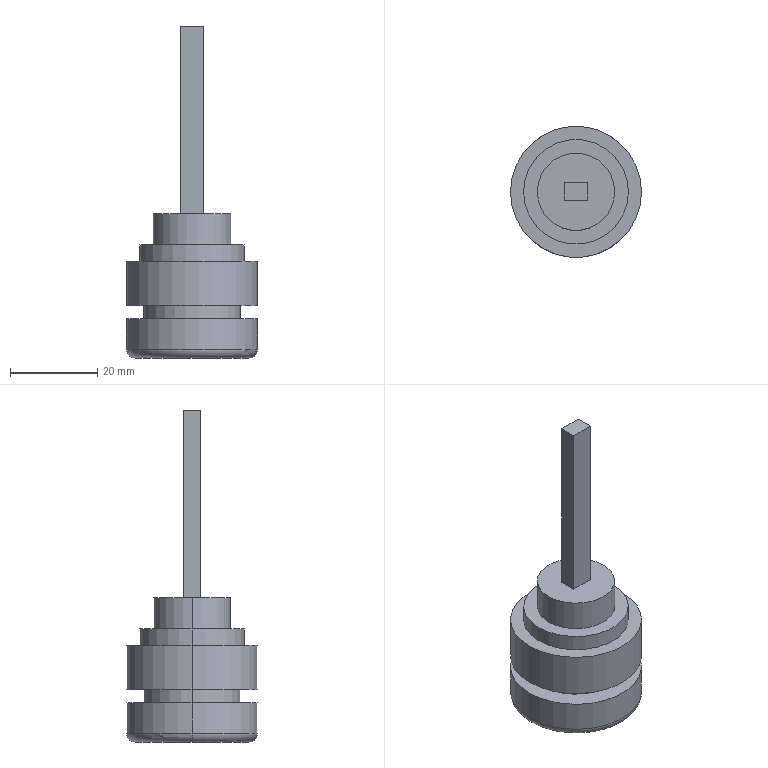Part | STEP file | Pushbutton head LA42PD-Y | 1 solid | 23 faces | box 30 x 30 x 76 mm | volume 18961 mm3 | plane 11 | cylinder 10 | torus 2 | commonest cylinder face diameters 30 x4 17.722 x2 22 x2 23.995 x2
STEP:
#1=CARTESIAN_POINT('',(0.,0.,0.));
#2=DIRECTION('',(0.,0.,1.));
#3=DIRECTION('',(1.,0.,0.));
#4=AXIS2_PLACEMENT_3D('',#1,#2,#3);
#5=CARTESIAN_POINT('',(13.,0.,0.));
#6=VERTEX_POINT('',#5);
#7=CARTESIAN_POINT('',(-13.,0.,0.));
#8=VERTEX_POINT('',#7);
#9=CARTESIAN_POINT('',(0.,0.,0.));
#10=DIRECTION('',(0.,0.,1.));
#11=DIRECTION('',(1.,0.,0.));
#12=AXIS2_PLACEMENT_3D('',#9,#10,#11);
#13=CIRCLE('',#12,13.);
#14=CARTESIAN_POINT('',(0.,0.,2.));
#15=DIRECTION('',(0.,0.,1.));
#16=DIRECTION('',(1.,0.,0.));
#17=AXIS2_PLACEMENT_3D('',#14,#15,#16);
#18=TOROIDAL_SURFACE('',#17,13.,2.);
#19=CARTESIAN_POINT('',(0.,4.712));
#20=DIRECTION('',(1.,0.));
#21=VECTOR('',#20,1.);
#22=LINE('',#19,#21);
#23=(GEOMETRIC_REPRESENTATION_CONTEXT(2)PARAMETRIC_REPRESENTATION_CONTEXT()REPRESENTATION_CONTEXT('',''));
#24=DEFINITIONAL_REPRESENTATION('',(#22),#23);
#25=PCURVE('',#18,#24);
#26=CARTESIAN_POINT('',(0.,0.,0.));
#27=DIRECTION('',(0.,0.,-1.));
#28=DIRECTION('',(-1.,0.,0.));
#29=AXIS2_PLACEMENT_3D('',#26,#27,#28);
#30=PLANE('',#29);
#31=CARTESIAN_POINT('',(-13.,0.));
#32=CARTESIAN_POINT('',(-13.,22.517));
#33=CARTESIAN_POINT('',(6.5,11.258));
#34=CARTESIAN_POINT('',(26.,0.));
#35=CARTESIAN_POINT('',(6.5,-11.258));
#36=CARTESIAN_POINT('',(-13.,-22.517));
#37=CARTESIAN_POINT('',(-13.,0.));
#38=(BOUNDED_CURVE()B_SPLINE_CURVE(2,(#31,#32,#33,#34,#35,#36,#37),.UNSPECIFIED.,.T.,.F.)B_SPLINE_CURVE_WITH_KNOTS((1,2,2,2,2,1),(-2.094,0.,2.094,4.189,6.283,8.378),.UNSPECIFIED.)CURVE()GEOMETRIC_REPRESENTATION_ITEM()RATIONAL_B_SPLINE_CURVE((1.,0.5,1.,0.5,1.,0.5,1.))REPRESENTATION_ITEM(''));
#39=(GEOMETRIC_REPRESENTATION_CONTEXT(2)PARAMETRIC_REPRESENTATION_CONTEXT()REPRESENTATION_CONTEXT('',''));
#40=DEFINITIONAL_REPRESENTATION('',(#38),#39);
#41=PCURVE('',#30,#40);
#42=SURFACE_CURVE('',#13,(#25,#41),.PCURVE_S1.);
#43=EDGE_CURVE('',#6,#8,#42,.T.);
#44=ORIENTED_EDGE('',*,*,#43,.T.);
#45=CARTESIAN_POINT('',(-15.,0.,2.));
#46=VERTEX_POINT('',#45);
#47=CARTESIAN_POINT('',(-13.,0.,2.));
#48=DIRECTION('',(0.,1.,0.));
#49=DIRECTION('',(-1.,0.,0.));
#50=AXIS2_PLACEMENT_3D('',#47,#48,#49);
#51=CIRCLE('',#50,2.);
#52=CARTESIAN_POINT('',(3.142,0.));
#53=DIRECTION('',(0.,1.));
#54=VECTOR('',#53,1.);
#55=LINE('',#52,#54);
#56=(GEOMETRIC_REPRESENTATION_CONTEXT(2)PARAMETRIC_REPRESENTATION_CONTEXT()REPRESENTATION_CONTEXT('',''));
#57=DEFINITIONAL_REPRESENTATION('',(#55),#56);
#58=PCURVE('',#18,#57);
#59=CARTESIAN_POINT('',(0.,0.,2.));
#60=DIRECTION('',(0.,0.,1.));
#61=DIRECTION('',(1.,0.,0.));
#62=AXIS2_PLACEMENT_3D('',#59,#60,#61);
#63=TOROIDAL_SURFACE('',#62,13.,2.);
#64=CARTESIAN_POINT('',(3.142,0.));
#65=DIRECTION('',(0.,1.));
#66=VECTOR('',#65,1.);
#67=LINE('',#64,#66);
#68=(GEOMETRIC_REPRESENTATION_CONTEXT(2)PARAMETRIC_REPRESENTATION_CONTEXT()REPRESENTATION_CONTEXT('',''));
#69=DEFINITIONAL_REPRESENTATION('',(#67),#68);
#70=PCURVE('',#63,#69);
#71=SURFACE_CURVE('',#51,(#58,#70),.PCURVE_S1.);
#72=EDGE_CURVE('',#8,#46,#71,.T.);
#73=ORIENTED_EDGE('',*,*,#72,.T.);
#74=CARTESIAN_POINT('',(15.,0.,2.));
#75=VERTEX_POINT('',#74);
#76=CARTESIAN_POINT('',(0.,0.,2.));
#77=DIRECTION('',(0.,0.,1.));
#78=DIRECTION('',(1.,0.,0.));
#79=AXIS2_PLACEMENT_3D('',#76,#77,#78);
#80=CIRCLE('',#79,15.);
#81=CARTESIAN_POINT('',(0.,6.283));
#82=DIRECTION('',(1.,0.));
#83=VECTOR('',#82,1.);
#84=LINE('',#81,#83);
#85=(GEOMETRIC_REPRESENTATION_CONTEXT(2)PARAMETRIC_REPRESENTATION_CONTEXT()REPRESENTATION_CONTEXT('',''));
#86=DEFINITIONAL_REPRESENTATION('',(#84),#85);
#87=PCURVE('',#18,#86);
#88=CARTESIAN_POINT('',(0.,0.,33.));
#89=DIRECTION('',(0.,0.,1.));
#90=DIRECTION('',(1.,0.,0.));
#91=AXIS2_PLACEMENT_3D('',#88,#89,#90);
#92=CYLINDRICAL_SURFACE('',#91,15.);
#93=CARTESIAN_POINT('',(0.,-31.));
#94=DIRECTION('',(1.,0.));
#95=VECTOR('',#94,1.);
#96=LINE('',#93,#95);
#97=(GEOMETRIC_REPRESENTATION_CONTEXT(2)PARAMETRIC_REPRESENTATION_CONTEXT()REPRESENTATION_CONTEXT('',''));
#98=DEFINITIONAL_REPRESENTATION('',(#96),#97);
#99=PCURVE('',#92,#98);
#100=SURFACE_CURVE('',#80,(#87,#99),.PCURVE_S1.);
#101=EDGE_CURVE('',#75,#46,#100,.T.);
#102=ORIENTED_EDGE('',*,*,#101,.F.);
#103=CARTESIAN_POINT('',(13.,0.,2.));
#104=DIRECTION('',(0.,-1.,0.));
#105=DIRECTION('',(0.,0.,-1.));
#106=AXIS2_PLACEMENT_3D('',#103,#104,#105);
#107=CIRCLE('',#106,2.);
#108=CARTESIAN_POINT('',(0.,4.712));
#109=DIRECTION('',(0.,1.));
#110=VECTOR('',#109,1.);
#111=LINE('',#108,#110);
#112=(GEOMETRIC_REPRESENTATION_CONTEXT(2)PARAMETRIC_REPRESENTATION_CONTEXT()REPRESENTATION_CONTEXT('',''));
#113=DEFINITIONAL_REPRESENTATION('',(#111),#112);
#114=PCURVE('',#18,#113);
#115=CARTESIAN_POINT('',(6.283,4.712));
#116=DIRECTION('',(0.,1.));
#117=VECTOR('',#116,1.);
#118=LINE('',#115,#117);
#119=(GEOMETRIC_REPRESENTATION_CONTEXT(2)PARAMETRIC_REPRESENTATION_CONTEXT()REPRESENTATION_CONTEXT('',''));
#120=DEFINITIONAL_REPRESENTATION('',(#118),#119);
#121=PCURVE('',#63,#120);
#122=SURFACE_CURVE('',#107,(#114,#121),.PCURVE_S1.);
#123=EDGE_CURVE('',#6,#75,#122,.T.);
#124=ORIENTED_EDGE('',*,*,#123,.F.);
#125=EDGE_LOOP('',(#44,#73,#102,#124));
#126=FACE_BOUND('',#125,.T.);
#127=ADVANCED_FACE('',(#126),#18,.T.);
#128=ORIENTED_EDGE('',*,*,#101,.T.);
#129=CARTESIAN_POINT('',(-15.,0.,9.));
#130=VERTEX_POINT('',#129);
#131=CARTESIAN_POINT('',(-15.,0.,33.));
#132=DIRECTION('',(0.,0.,1.));
#133=VECTOR('',#132,1.);
#134=LINE('',#131,#133);
#135=CARTESIAN_POINT('',(3.142,0.));
#136=DIRECTION('',(0.,1.));
#137=VECTOR('',#136,1.);
#138=LINE('',#135,#137);
#139=(GEOMETRIC_REPRESENTATION_CONTEXT(2)PARAMETRIC_REPRESENTATION_CONTEXT()REPRESENTATION_CONTEXT('',''));
#140=DEFINITIONAL_REPRESENTATION('',(#138),#139);
#141=PCURVE('',#92,#140);
#142=CARTESIAN_POINT('',(0.,0.,33.));
#143=DIRECTION('',(0.,0.,1.));
#144=DIRECTION('',(1.,0.,0.));
#145=AXIS2_PLACEMENT_3D('',#142,#143,#144);
#146=CYLINDRICAL_SURFACE('',#145,15.);
#147=CARTESIAN_POINT('',(3.142,0.));
#148=DIRECTION('',(0.,1.));
#149=VECTOR('',#148,1.);
#150=LINE('',#147,#149);
#151=(GEOMETRIC_REPRESENTATION_CONTEXT(2)PARAMETRIC_REPRESENTATION_CONTEXT()REPRESENTATION_CONTEXT('',''));
#152=DEFINITIONAL_REPRESENTATION('',(#150),#151);
#153=PCURVE('',#146,#152);
#154=SURFACE_CURVE('',#134,(#141,#153),.PCURVE_S1.);
#155=EDGE_CURVE('',#46,#130,#154,.T.);
#156=ORIENTED_EDGE('',*,*,#155,.T.);
#157=CARTESIAN_POINT('',(15.,0.,9.));
#158=VERTEX_POINT('',#157);
#159=CARTESIAN_POINT('',(0.,0.,9.));
#160=DIRECTION('',(0.,0.,1.));
#161=DIRECTION('',(1.,0.,0.));
#162=AXIS2_PLACEMENT_3D('',#159,#160,#161);
#163=CIRCLE('',#162,15.);
#164=CARTESIAN_POINT('',(0.,-24.));
#165=DIRECTION('',(1.,0.));
#166=VECTOR('',#165,1.);
#167=LINE('',#164,#166);
#168=(GEOMETRIC_REPRESENTATION_CONTEXT(2)PARAMETRIC_REPRESENTATION_CONTEXT()REPRESENTATION_CONTEXT('',''));
#169=DEFINITIONAL_REPRESENTATION('',(#167),#168);
#170=PCURVE('',#92,#169);
#171=CARTESIAN_POINT('',(15.,0.,9.));
#172=DIRECTION('',(0.,0.,1.));
#173=DIRECTION('',(1.,0.,0.));
#174=AXIS2_PLACEMENT_3D('',#171,#172,#173);
#175=PLANE('',#174);
#176=CARTESIAN_POINT('',(-15.,0.));
#177=DIRECTION('',(1.,0.));
#178=AXIS2_PLACEMENT_2D('',#176,#177);
#179=CIRCLE('',#178,15.);
#180=(GEOMETRIC_REPRESENTATION_CONTEXT(2)PARAMETRIC_REPRESENTATION_CONTEXT()REPRESENTATION_CONTEXT('',''));
#181=DEFINITIONAL_REPRESENTATION('',(#179),#180);
#182=PCURVE('',#175,#181);
#183=SURFACE_CURVE('',#163,(#170,#182),.PCURVE_S1.);
#184=EDGE_CURVE('',#158,#130,#183,.T.);
#185=ORIENTED_EDGE('',*,*,#184,.F.);
#186=CARTESIAN_POINT('',(15.,0.,33.));
#187=DIRECTION('',(0.,0.,1.));
#188=VECTOR('',#187,1.);
#189=LINE('',#186,#188);
#190=CARTESIAN_POINT('',(0.,0.));
#191=DIRECTION('',(0.,1.));
#192=VECTOR('',#191,1.);
#193=LINE('',#190,#192);
#194=(GEOMETRIC_REPRESENTATION_CONTEXT(2)PARAMETRIC_REPRESENTATION_CONTEXT()REPRESENTATION_CONTEXT('',''));
#195=DEFINITIONAL_REPRESENTATION('',(#193),#194);
#196=PCURVE('',#92,#195);
#197=CARTESIAN_POINT('',(6.283,0.));
#198=DIRECTION('',(0.,1.));
#199=VECTOR('',#198,1.);
#200=LINE('',#197,#199);
#201=(GEOMETRIC_REPRESENTATION_CONTEXT(2)PARAMETRIC_REPRESENTATION_CONTEXT()REPRESENTATION_CONTEXT('',''));
#202=DEFINITIONAL_REPRESENTATION('',(#200),#201);
#203=PCURVE('',#146,#202);
#204=SURFACE_CURVE('',#189,(#196,#203),.PCURVE_S1.);
#205=EDGE_CURVE('',#75,#158,#204,.T.);
#206=ORIENTED_EDGE('',*,*,#205,.F.);
#207=EDGE_LOOP('',(#128,#156,#185,#206));
#208=FACE_BOUND('',#207,.T.);
#209=ADVANCED_FACE('',(#208),#92,.T.);
#210=CARTESIAN_POINT('',(11.,0.,9.));
#211=VERTEX_POINT('',#210);
#212=CARTESIAN_POINT('',(-11.,0.,9.));
#213=VERTEX_POINT('',#212);
#214=CARTESIAN_POINT('',(0.,0.,9.));
#215=DIRECTION('',(0.,0.,1.));
#216=DIRECTION('',(1.,0.,0.));
#217=AXIS2_PLACEMENT_3D('',#214,#215,#216);
#218=CIRCLE('',#217,11.);
#219=CARTESIAN_POINT('',(0.,0.,33.));
#220=DIRECTION('',(0.,0.,1.));
#221=DIRECTION('',(1.,0.,0.));
#222=AXIS2_PLACEMENT_3D('',#219,#220,#221);
#223=CYLINDRICAL_SURFACE('',#222,11.);
#224=CARTESIAN_POINT('',(0.,-24.));
#225=DIRECTION('',(1.,0.));
#226=VECTOR('',#225,1.);
#227=LINE('',#224,#226);
#228=(GEOMETRIC_REPRESENTATION_CONTEXT(2)PARAMETRIC_REPRESENTATION_CONTEXT()REPRESENTATION_CONTEXT('',''));
#229=DEFINITIONAL_REPRESENTATION('',(#227),#228);
#230=PCURVE('',#223,#229);
#231=CARTESIAN_POINT('',(-15.,0.));
#232=DIRECTION('',(1.,0.));
#233=AXIS2_PLACEMENT_2D('',#231,#232);
#234=CIRCLE('',#233,11.);
#235=(GEOMETRIC_REPRESENTATION_CONTEXT(2)PARAMETRIC_REPRESENTATION_CONTEXT()REPRESENTATION_CONTEXT('',''));
#236=DEFINITIONAL_REPRESENTATION('',(#234),#235);
#237=PCURVE('',#175,#236);
#238=SURFACE_CURVE('',#218,(#230,#237),.PCURVE_S1.);
#239=EDGE_CURVE('',#211,#213,#238,.T.);
#240=ORIENTED_EDGE('',*,*,#239,.T.);
#241=CARTESIAN_POINT('',(-11.,0.,12.));
#242=VERTEX_POINT('',#241);
#243=CARTESIAN_POINT('',(-11.,0.,33.));
#244=DIRECTION('',(0.,0.,1.));
#245=VECTOR('',#244,1.);
#246=LINE('',#243,#245);
#247=CARTESIAN_POINT('',(3.142,0.));
#248=DIRECTION('',(0.,1.));
#249=VECTOR('',#248,1.);
#250=LINE('',#247,#249);
#251=(GEOMETRIC_REPRESENTATION_CONTEXT(2)PARAMETRIC_REPRESENTATION_CONTEXT()REPRESENTATION_CONTEXT('',''));
#252=DEFINITIONAL_REPRESENTATION('',(#250),#251);
#253=PCURVE('',#223,#252);
#254=CARTESIAN_POINT('',(0.,0.,33.));
#255=DIRECTION('',(0.,0.,1.));
#256=DIRECTION('',(1.,0.,0.));
#257=AXIS2_PLACEMENT_3D('',#254,#255,#256);
#258=CYLINDRICAL_SURFACE('',#257,11.);
#259=CARTESIAN_POINT('',(3.142,0.));
#260=DIRECTION('',(0.,1.));
#261=VECTOR('',#260,1.);
#262=LINE('',#259,#261);
#263=(GEOMETRIC_REPRESENTATION_CONTEXT(2)PARAMETRIC_REPRESENTATION_CONTEXT()REPRESENTATION_CONTEXT('',''));
#264=DEFINITIONAL_REPRESENTATION('',(#262),#263);
#265=PCURVE('',#258,#264);
#266=SURFACE_CURVE('',#246,(#253,#265),.PCURVE_S1.);
#267=EDGE_CURVE('',#213,#242,#266,.T.);
#268=ORIENTED_EDGE('',*,*,#267,.T.);
#269=CARTESIAN_POINT('',(11.,0.,12.));
#270=VERTEX_POINT('',#269);
#271=CARTESIAN_POINT('',(0.,0.,12.));
#272=DIRECTION('',(0.,0.,1.));
#273=DIRECTION('',(1.,0.,0.));
#274=AXIS2_PLACEMENT_3D('',#271,#272,#273);
#275=CIRCLE('',#274,11.);
#276=CARTESIAN_POINT('',(0.,-21.));
#277=DIRECTION('',(1.,0.));
#278=VECTOR('',#277,1.);
#279=LINE('',#276,#278);
#280=(GEOMETRIC_REPRESENTATION_CONTEXT(2)PARAMETRIC_REPRESENTATION_CONTEXT()REPRESENTATION_CONTEXT('',''));
#281=DEFINITIONAL_REPRESENTATION('',(#279),#280);
#282=PCURVE('',#223,#281);
#283=CARTESIAN_POINT('',(11.,0.,12.));
#284=DIRECTION('',(0.,0.,-1.));
#285=DIRECTION('',(-1.,0.,0.));
#286=AXIS2_PLACEMENT_3D('',#283,#284,#285);
#287=PLANE('',#286);
#288=CARTESIAN_POINT('',(0.,0.));
#289=CARTESIAN_POINT('',(0.,19.053));
#290=CARTESIAN_POINT('',(16.5,9.526));
#291=CARTESIAN_POINT('',(33.,0.));
#292=CARTESIAN_POINT('',(16.5,-9.526));
#293=CARTESIAN_POINT('',(0.,-19.053));
#294=CARTESIAN_POINT('',(0.,0.));
#295=(BOUNDED_CURVE()B_SPLINE_CURVE(2,(#288,#289,#290,#291,#292,#293,#294),.UNSPECIFIED.,.T.,.F.)B_SPLINE_CURVE_WITH_KNOTS((1,2,2,2,2,1),(-2.094,0.,2.094,4.189,6.283,8.378),.UNSPECIFIED.)CURVE()GEOMETRIC_REPRESENTATION_ITEM()RATIONAL_B_SPLINE_CURVE((1.,0.5,1.,0.5,1.,0.5,1.))REPRESENTATION_ITEM(''));
#296=(GEOMETRIC_REPRESENTATION_CONTEXT(2)PARAMETRIC_REPRESENTATION_CONTEXT()REPRESENTATION_CONTEXT('',''));
#297=DEFINITIONAL_REPRESENTATION('',(#295),#296);
#298=PCURVE('',#287,#297);
#299=SURFACE_CURVE('',#275,(#282,#298),.PCURVE_S1.);
#300=EDGE_CURVE('',#270,#242,#299,.T.);
#301=ORIENTED_EDGE('',*,*,#300,.F.);
#302=CARTESIAN_POINT('',(11.,0.,33.));
#303=DIRECTION('',(0.,0.,1.));
#304=VECTOR('',#303,1.);
#305=LINE('',#302,#304);
#306=CARTESIAN_POINT('',(0.,0.));
#307=DIRECTION('',(0.,1.));
#308=VECTOR('',#307,1.);
#309=LINE('',#306,#308);
#310=(GEOMETRIC_REPRESENTATION_CONTEXT(2)PARAMETRIC_REPRESENTATION_CONTEXT()REPRESENTATION_CONTEXT('',''));
#311=DEFINITIONAL_REPRESENTATION('',(#309),#310);
#312=PCURVE('',#223,#311);
#313=CARTESIAN_POINT('',(6.283,0.));
#314=DIRECTION('',(0.,1.));
#315=VECTOR('',#314,1.);
#316=LINE('',#313,#315);
#317=(GEOMETRIC_REPRESENTATION_CONTEXT(2)PARAMETRIC_REPRESENTATION_CONTEXT()REPRESENTATION_CONTEXT('',''));
#318=DEFINITIONAL_REPRESENTATION('',(#316),#317);
#319=PCURVE('',#258,#318);
#320=SURFACE_CURVE('',#305,(#312,#319),.PCURVE_S1.);
#321=EDGE_CURVE('',#211,#270,#320,.T.);
#322=ORIENTED_EDGE('',*,*,#321,.F.);
#323=EDGE_LOOP('',(#240,#268,#301,#322));
#324=FACE_BOUND('',#323,.T.);
#325=ADVANCED_FACE('',(#324),#223,.T.);
#326=CARTESIAN_POINT('',(15.,0.,12.));
#327=VERTEX_POINT('',#326);
#328=CARTESIAN_POINT('',(-15.,0.,12.));
#329=VERTEX_POINT('',#328);
#330=CARTESIAN_POINT('',(0.,0.,12.));
#331=DIRECTION('',(0.,0.,1.));
#332=DIRECTION('',(1.,0.,0.));
#333=AXIS2_PLACEMENT_3D('',#330,#331,#332);
#334=CIRCLE('',#333,15.);
#335=CARTESIAN_POINT('',(0.,0.,33.));
#336=DIRECTION('',(0.,0.,1.));
#337=DIRECTION('',(1.,0.,0.));
#338=AXIS2_PLACEMENT_3D('',#335,#336,#337);
#339=CYLINDRICAL_SURFACE('',#338,15.);
#340=CARTESIAN_POINT('',(0.,-21.));
#341=DIRECTION('',(1.,0.));
#342=VECTOR('',#341,1.);
#343=LINE('',#340,#342);
#344=(GEOMETRIC_REPRESENTATION_CONTEXT(2)PARAMETRIC_REPRESENTATION_CONTEXT()REPRESENTATION_CONTEXT('',''));
#345=DEFINITIONAL_REPRESENTATION('',(#343),#344);
#346=PCURVE('',#339,#345);
#347=CARTESIAN_POINT('',(-4.,0.));
#348=CARTESIAN_POINT('',(-4.,25.981));
#349=CARTESIAN_POINT('',(18.5,12.99));
#350=CARTESIAN_POINT('',(41.,0.));
#351=CARTESIAN_POINT('',(18.5,-12.99));
#352=CARTESIAN_POINT('',(-4.,-25.981));
#353=CARTESIAN_POINT('',(-4.,0.));
#354=(BOUNDED_CURVE()B_SPLINE_CURVE(2,(#347,#348,#349,#350,#351,#352,#353),.UNSPECIFIED.,.T.,.F.)B_SPLINE_CURVE_WITH_KNOTS((1,2,2,2,2,1),(-2.094,0.,2.094,4.189,6.283,8.378),.UNSPECIFIED.)CURVE()GEOMETRIC_REPRESENTATION_ITEM()RATIONAL_B_SPLINE_CURVE((1.,0.5,1.,0.5,1.,0.5,1.))REPRESENTATION_ITEM(''));
#355=(GEOMETRIC_REPRESENTATION_CONTEXT(2)PARAMETRIC_REPRESENTATION_CONTEXT()REPRESENTATION_CONTEXT('',''));
#356=DEFINITIONAL_REPRESENTATION('',(#354),#355);
#357=PCURVE('',#287,#356);
#358=SURFACE_CURVE('',#334,(#346,#357),.PCURVE_S1.);
#359=EDGE_CURVE('',#327,#329,#358,.T.);
#360=ORIENTED_EDGE('',*,*,#359,.T.);
#361=CARTESIAN_POINT('',(-15.,0.,22.166));
#362=VERTEX_POINT('',#361);
#363=CARTESIAN_POINT('',(-15.,0.,33.));
#364=DIRECTION('',(0.,0.,1.));
#365=VECTOR('',#364,1.);
#366=LINE('',#363,#365);
#367=CARTESIAN_POINT('',(3.142,0.));
#368=DIRECTION('',(0.,1.));
#369=VECTOR('',#368,1.);
#370=LINE('',#367,#369);
#371=(GEOMETRIC_REPRESENTATION_CONTEXT(2)PARAMETRIC_REPRESENTATION_CONTEXT()REPRESENTATION_CONTEXT('',''));
#372=DEFINITIONAL_REPRESENTATION('',(#370),#371);
#373=PCURVE('',#339,#372);
#374=CARTESIAN_POINT('',(0.,0.,33.));
#375=DIRECTION('',(0.,0.,1.));
#376=DIRECTION('',(1.,0.,0.));
#377=AXIS2_PLACEMENT_3D('',#374,#375,#376);
#378=CYLINDRICAL_SURFACE('',#377,15.);
#379=CARTESIAN_POINT('',(3.142,0.));
#380=DIRECTION('',(0.,1.));
#381=VECTOR('',#380,1.);
#382=LINE('',#379,#381);
#383=(GEOMETRIC_REPRESENTATION_CONTEXT(2)PARAMETRIC_REPRESENTATION_CONTEXT()REPRESENTATION_CONTEXT('',''));
#384=DEFINITIONAL_REPRESENTATION('',(#382),#383);
#385=PCURVE('',#378,#384);
#386=SURFACE_CURVE('',#366,(#373,#385),.PCURVE_S1.);
#387=EDGE_CURVE('',#329,#362,#386,.T.);
#388=ORIENTED_EDGE('',*,*,#387,.T.);
#389=CARTESIAN_POINT('',(15.,0.,22.166));
#390=VERTEX_POINT('',#389);
#391=CARTESIAN_POINT('',(0.,0.,22.166));
#392=DIRECTION('',(0.,0.,1.));
#393=DIRECTION('',(1.,0.,0.));
#394=AXIS2_PLACEMENT_3D('',#391,#392,#393);
#395=CIRCLE('',#394,15.);
#396=CARTESIAN_POINT('',(0.,-10.834));
#397=DIRECTION('',(1.,0.));
#398=VECTOR('',#397,1.);
#399=LINE('',#396,#398);
#400=(GEOMETRIC_REPRESENTATION_CONTEXT(2)PARAMETRIC_REPRESENTATION_CONTEXT()REPRESENTATION_CONTEXT('',''));
#401=DEFINITIONAL_REPRESENTATION('',(#399),#400);
#402=PCURVE('',#339,#401);
#403=CARTESIAN_POINT('',(15.,0.,22.166));
#404=DIRECTION('',(0.,0.,1.));
#405=DIRECTION('',(1.,0.,0.));
#406=AXIS2_PLACEMENT_3D('',#403,#404,#405);
#407=PLANE('',#406);
#408=CARTESIAN_POINT('',(-15.,0.));
#409=DIRECTION('',(1.,0.));
#410=AXIS2_PLACEMENT_2D('',#408,#409);
#411=CIRCLE('',#410,15.);
#412=(GEOMETRIC_REPRESENTATION_CONTEXT(2)PARAMETRIC_REPRESENTATION_CONTEXT()REPRESENTATION_CONTEXT('',''));
#413=DEFINITIONAL_REPRESENTATION('',(#411),#412);
#414=PCURVE('',#407,#413);
#415=SURFACE_CURVE('',#395,(#402,#414),.PCURVE_S1.);
#416=EDGE_CURVE('',#390,#362,#415,.T.);
#417=ORIENTED_EDGE('',*,*,#416,.F.);
#418=CARTESIAN_POINT('',(15.,0.,33.));
#419=DIRECTION('',(0.,0.,1.));
#420=VECTOR('',#419,1.);
#421=LINE('',#418,#420);
#422=CARTESIAN_POINT('',(0.,0.));
#423=DIRECTION('',(0.,1.));
#424=VECTOR('',#423,1.);
#425=LINE('',#422,#424);
#426=(GEOMETRIC_REPRESENTATION_CONTEXT(2)PARAMETRIC_REPRESENTATION_CONTEXT()REPRESENTATION_CONTEXT('',''));
#427=DEFINITIONAL_REPRESENTATION('',(#425),#426);
#428=PCURVE('',#339,#427);
#429=CARTESIAN_POINT('',(6.283,0.));
#430=DIRECTION('',(0.,1.));
#431=VECTOR('',#430,1.);
#432=LINE('',#429,#431);
#433=(GEOMETRIC_REPRESENTATION_CONTEXT(2)PARAMETRIC_REPRESENTATION_CONTEXT()REPRESENTATION_CONTEXT('',''));
#434=DEFINITIONAL_REPRESENTATION('',(#432),#433);
#435=PCURVE('',#378,#434);
#436=SURFACE_CURVE('',#421,(#428,#435),.PCURVE_S1.);
#437=EDGE_CURVE('',#327,#390,#436,.T.);
#438=ORIENTED_EDGE('',*,*,#437,.F.);
#439=EDGE_LOOP('',(#360,#388,#417,#438));
#440=FACE_BOUND('',#439,.T.);
#441=ADVANCED_FACE('',(#440),#339,.T.);
#442=CARTESIAN_POINT('',(11.997,0.,22.166));
#443=VERTEX_POINT('',#442);
#444=CARTESIAN_POINT('',(-11.997,0.,22.166));
#445=VERTEX_POINT('',#444);
#446=CARTESIAN_POINT('',(0.,0.,22.166));
#447=DIRECTION('',(0.,0.,1.));
#448=DIRECTION('',(1.,0.,0.));
#449=AXIS2_PLACEMENT_3D('',#446,#447,#448);
#450=CIRCLE('',#449,11.997);
#451=CARTESIAN_POINT('',(0.,0.,33.));
#452=DIRECTION('',(0.,0.,1.));
#453=DIRECTION('',(1.,0.,0.));
#454=AXIS2_PLACEMENT_3D('',#451,#452,#453);
#455=CYLINDRICAL_SURFACE('',#454,11.997);
#456=CARTESIAN_POINT('',(0.,-10.834));
#457=DIRECTION('',(1.,0.));
#458=VECTOR('',#457,1.);
#459=LINE('',#456,#458);
#460=(GEOMETRIC_REPRESENTATION_CONTEXT(2)PARAMETRIC_REPRESENTATION_CONTEXT()REPRESENTATION_CONTEXT('',''));
#461=DEFINITIONAL_REPRESENTATION('',(#459),#460);
#462=PCURVE('',#455,#461);
#463=CARTESIAN_POINT('',(-15.,0.));
#464=DIRECTION('',(1.,0.));
#465=AXIS2_PLACEMENT_2D('',#463,#464);
#466=CIRCLE('',#465,11.997);
#467=(GEOMETRIC_REPRESENTATION_CONTEXT(2)PARAMETRIC_REPRESENTATION_CONTEXT()REPRESENTATION_CONTEXT('',''));
#468=DEFINITIONAL_REPRESENTATION('',(#466),#467);
#469=PCURVE('',#407,#468);
#470=SURFACE_CURVE('',#450,(#462,#469),.PCURVE_S1.);
#471=EDGE_CURVE('',#443,#445,#470,.T.);
#472=ORIENTED_EDGE('',*,*,#471,.T.);
#473=CARTESIAN_POINT('',(-11.997,0.,25.869));
#474=VERTEX_POINT('',#473);
#475=CARTESIAN_POINT('',(-11.997,0.,33.));
#476=DIRECTION('',(0.,0.,1.));
#477=VECTOR('',#476,1.);
#478=LINE('',#475,#477);
#479=CARTESIAN_POINT('',(3.142,0.));
#480=DIRECTION('',(0.,1.));
#481=VECTOR('',#480,1.);
#482=LINE('',#479,#481);
#483=(GEOMETRIC_REPRESENTATION_CONTEXT(2)PARAMETRIC_REPRESENTATION_CONTEXT()REPRESENTATION_CONTEXT('',''));
#484=DEFINITIONAL_REPRESENTATION('',(#482),#483);
#485=PCURVE('',#455,#484);
#486=CARTESIAN_POINT('',(0.,0.,33.));
#487=DIRECTION('',(0.,0.,1.));
#488=DIRECTION('',(1.,0.,0.));
#489=AXIS2_PLACEMENT_3D('',#486,#487,#488);
#490=CYLINDRICAL_SURFACE('',#489,11.997);
#491=CARTESIAN_POINT('',(3.142,0.));
#492=DIRECTION('',(0.,1.));
#493=VECTOR('',#492,1.);
#494=LINE('',#491,#493);
#495=(GEOMETRIC_REPRESENTATION_CONTEXT(2)PARAMETRIC_REPRESENTATION_CONTEXT()REPRESENTATION_CONTEXT('',''));
#496=DEFINITIONAL_REPRESENTATION('',(#494),#495);
#497=PCURVE('',#490,#496);
#498=SURFACE_CURVE('',#478,(#485,#497),.PCURVE_S1.);
#499=EDGE_CURVE('',#445,#474,#498,.T.);
#500=ORIENTED_EDGE('',*,*,#499,.T.);
#501=CARTESIAN_POINT('',(11.997,0.,25.869));
#502=VERTEX_POINT('',#501);
#503=CARTESIAN_POINT('',(0.,0.,25.869));
#504=DIRECTION('',(0.,0.,1.));
#505=DIRECTION('',(1.,0.,0.));
#506=AXIS2_PLACEMENT_3D('',#503,#504,#505);
#507=CIRCLE('',#506,11.997);
#508=CARTESIAN_POINT('',(0.,-7.131));
#509=DIRECTION('',(1.,0.));
#510=VECTOR('',#509,1.);
#511=LINE('',#508,#510);
#512=(GEOMETRIC_REPRESENTATION_CONTEXT(2)PARAMETRIC_REPRESENTATION_CONTEXT()REPRESENTATION_CONTEXT('',''));
#513=DEFINITIONAL_REPRESENTATION('',(#511),#512);
#514=PCURVE('',#455,#513);
#515=CARTESIAN_POINT('',(11.997,0.,25.869));
#516=DIRECTION('',(0.,0.,1.));
#517=DIRECTION('',(1.,0.,0.));
#518=AXIS2_PLACEMENT_3D('',#515,#516,#517);
#519=PLANE('',#518);
#520=CARTESIAN_POINT('',(-11.997,0.));
#521=DIRECTION('',(1.,0.));
#522=AXIS2_PLACEMENT_2D('',#520,#521);
#523=CIRCLE('',#522,11.997);
#524=(GEOMETRIC_REPRESENTATION_CONTEXT(2)PARAMETRIC_REPRESENTATION_CONTEXT()REPRESENTATION_CONTEXT('',''));
#525=DEFINITIONAL_REPRESENTATION('',(#523),#524);
#526=PCURVE('',#519,#525);
#527=SURFACE_CURVE('',#507,(#514,#526),.PCURVE_S1.);
#528=EDGE_CURVE('',#502,#474,#527,.T.);
#529=ORIENTED_EDGE('',*,*,#528,.F.);
#530=CARTESIAN_POINT('',(11.997,0.,33.));
#531=DIRECTION('',(0.,0.,1.));
#532=VECTOR('',#531,1.);
#533=LINE('',#530,#532);
#534=CARTESIAN_POINT('',(0.,0.));
#535=DIRECTION('',(0.,1.));
#536=VECTOR('',#535,1.);
#537=LINE('',#534,#536);
#538=(GEOMETRIC_REPRESENTATION_CONTEXT(2)PARAMETRIC_REPRESENTATION_CONTEXT()REPRESENTATION_CONTEXT('',''));
#539=DEFINITIONAL_REPRESENTATION('',(#537),#538);
#540=PCURVE('',#455,#539);
#541=CARTESIAN_POINT('',(6.283,0.));
#542=DIRECTION('',(0.,1.));
#543=VECTOR('',#542,1.);
#544=LINE('',#541,#543);
#545=(GEOMETRIC_REPRESENTATION_CONTEXT(2)PARAMETRIC_REPRESENTATION_CONTEXT()REPRESENTATION_CONTEXT('',''));
#546=DEFINITIONAL_REPRESENTATION('',(#544),#545);
#547=PCURVE('',#490,#546);
#548=SURFACE_CURVE('',#533,(#540,#547),.PCURVE_S1.);
#549=EDGE_CURVE('',#443,#502,#548,.T.);
#550=ORIENTED_EDGE('',*,*,#549,.F.);
#551=EDGE_LOOP('',(#472,#500,#529,#550));
#552=FACE_BOUND('',#551,.T.);
#553=ADVANCED_FACE('',(#552),#455,.T.);
#554=CARTESIAN_POINT('',(8.861,0.,25.869));
#555=VERTEX_POINT('',#554);
#556=CARTESIAN_POINT('',(-8.861,0.,25.869));
#557=VERTEX_POINT('',#556);
#558=CARTESIAN_POINT('',(0.,0.,25.869));
#559=DIRECTION('',(0.,0.,1.));
#560=DIRECTION('',(1.,0.,0.));
#561=AXIS2_PLACEMENT_3D('',#558,#559,#560);
#562=CIRCLE('',#561,8.861);
#563=CARTESIAN_POINT('',(0.,0.,33.));
#564=DIRECTION('',(0.,0.,1.));
#565=DIRECTION('',(1.,0.,0.));
#566=AXIS2_PLACEMENT_3D('',#563,#564,#565);
#567=CYLINDRICAL_SURFACE('',#566,8.861);
#568=CARTESIAN_POINT('',(0.,-7.131));
#569=DIRECTION('',(1.,0.));
#570=VECTOR('',#569,1.);
#571=LINE('',#568,#570);
#572=(GEOMETRIC_REPRESENTATION_CONTEXT(2)PARAMETRIC_REPRESENTATION_CONTEXT()REPRESENTATION_CONTEXT('',''));
#573=DEFINITIONAL_REPRESENTATION('',(#571),#572);
#574=PCURVE('',#567,#573);
#575=CARTESIAN_POINT('',(-11.997,0.));
#576=DIRECTION('',(1.,0.));
#577=AXIS2_PLACEMENT_2D('',#575,#576);
#578=CIRCLE('',#577,8.861);
#579=(GEOMETRIC_REPRESENTATION_CONTEXT(2)PARAMETRIC_REPRESENTATION_CONTEXT()REPRESENTATION_CONTEXT('',''));
#580=DEFINITIONAL_REPRESENTATION('',(#578),#579);
#581=PCURVE('',#519,#580);
#582=SURFACE_CURVE('',#562,(#574,#581),.PCURVE_S1.);
#583=EDGE_CURVE('',#555,#557,#582,.T.);
#584=ORIENTED_EDGE('',*,*,#583,.T.);
#585=CARTESIAN_POINT('',(-8.861,0.,33.));
#586=VERTEX_POINT('',#585);
#587=CARTESIAN_POINT('',(-8.861,0.,33.));
#588=DIRECTION('',(0.,0.,1.));
#589=VECTOR('',#588,1.);
#590=LINE('',#587,#589);
#591=CARTESIAN_POINT('',(3.142,0.));
#592=DIRECTION('',(0.,1.));
#593=VECTOR('',#592,1.);
#594=LINE('',#591,#593);
#595=(GEOMETRIC_REPRESENTATION_CONTEXT(2)PARAMETRIC_REPRESENTATION_CONTEXT()REPRESENTATION_CONTEXT('',''));
#596=DEFINITIONAL_REPRESENTATION('',(#594),#595);
#597=PCURVE('',#567,#596);
#598=CARTESIAN_POINT('',(0.,0.,33.));
#599=DIRECTION('',(0.,0.,1.));
#600=DIRECTION('',(1.,0.,0.));
#601=AXIS2_PLACEMENT_3D('',#598,#599,#600);
#602=CYLINDRICAL_SURFACE('',#601,8.861);
#603=CARTESIAN_POINT('',(3.142,0.));
#604=DIRECTION('',(0.,1.));
#605=VECTOR('',#604,1.);
#606=LINE('',#603,#605);
#607=(GEOMETRIC_REPRESENTATION_CONTEXT(2)PARAMETRIC_REPRESENTATION_CONTEXT()REPRESENTATION_CONTEXT('',''));
#608=DEFINITIONAL_REPRESENTATION('',(#606),#607);
#609=PCURVE('',#602,#608);
#610=SURFACE_CURVE('',#590,(#597,#609),.PCURVE_S1.);
#611=EDGE_CURVE('',#557,#586,#610,.T.);
#612=ORIENTED_EDGE('',*,*,#611,.T.);
#613=CARTESIAN_POINT('',(8.861,0.,33.));
#614=VERTEX_POINT('',#613);
#615=CARTESIAN_POINT('',(0.,0.,33.));
#616=DIRECTION('',(0.,0.,1.));
#617=DIRECTION('',(1.,0.,0.));
#618=AXIS2_PLACEMENT_3D('',#615,#616,#617);
#619=CIRCLE('',#618,8.861);
#620=CARTESIAN_POINT('',(0.,0.));
#621=DIRECTION('',(1.,0.));
#622=VECTOR('',#621,1.);
#623=LINE('',#620,#622);
#624=(GEOMETRIC_REPRESENTATION_CONTEXT(2)PARAMETRIC_REPRESENTATION_CONTEXT()REPRESENTATION_CONTEXT('',''));
#625=DEFINITIONAL_REPRESENTATION('',(#623),#624);
#626=PCURVE('',#567,#625);
#627=CARTESIAN_POINT('',(8.861,0.,33.));
#628=DIRECTION('',(0.,0.,1.));
#629=DIRECTION('',(1.,0.,0.));
#630=AXIS2_PLACEMENT_3D('',#627,#628,#629);
#631=PLANE('',#630);
#632=CARTESIAN_POINT('',(-8.861,0.));
#633=DIRECTION('',(1.,0.));
#634=AXIS2_PLACEMENT_2D('',#632,#633);
#635=CIRCLE('',#634,8.861);
#636=(GEOMETRIC_REPRESENTATION_CONTEXT(2)PARAMETRIC_REPRESENTATION_CONTEXT()REPRESENTATION_CONTEXT('',''));
#637=DEFINITIONAL_REPRESENTATION('',(#635),#636);
#638=PCURVE('',#631,#637);
#639=SURFACE_CURVE('',#619,(#626,#638),.PCURVE_S1.);
#640=EDGE_CURVE('',#614,#586,#639,.T.);
#641=ORIENTED_EDGE('',*,*,#640,.F.);
#642=CARTESIAN_POINT('',(8.861,0.,33.));
#643=DIRECTION('',(0.,0.,1.));
#644=VECTOR('',#643,1.);
#645=LINE('',#642,#644);
#646=CARTESIAN_POINT('',(0.,0.));
#647=DIRECTION('',(0.,1.));
#648=VECTOR('',#647,1.);
#649=LINE('',#646,#648);
#650=(GEOMETRIC_REPRESENTATION_CONTEXT(2)PARAMETRIC_REPRESENTATION_CONTEXT()REPRESENTATION_CONTEXT('',''));
#651=DEFINITIONAL_REPRESENTATION('',(#649),#650);
#652=PCURVE('',#567,#651);
#653=CARTESIAN_POINT('',(6.283,0.));
#654=DIRECTION('',(0.,1.));
#655=VECTOR('',#654,1.);
#656=LINE('',#653,#655);
#657=(GEOMETRIC_REPRESENTATION_CONTEXT(2)PARAMETRIC_REPRESENTATION_CONTEXT()REPRESENTATION_CONTEXT('',''));
#658=DEFINITIONAL_REPRESENTATION('',(#656),#657);
#659=PCURVE('',#602,#658);
#660=SURFACE_CURVE('',#645,(#652,#659),.PCURVE_S1.);
#661=EDGE_CURVE('',#555,#614,#660,.T.);
#662=ORIENTED_EDGE('',*,*,#661,.F.);
#663=EDGE_LOOP('',(#584,#612,#641,#662));
#664=FACE_BOUND('',#663,.T.);
#665=ADVANCED_FACE('',(#664),#567,.T.);
#666=ORIENTED_EDGE('',*,*,#640,.T.);
#667=CARTESIAN_POINT('',(0.,0.,33.));
#668=DIRECTION('',(0.,0.,1.));
#669=DIRECTION('',(1.,0.,0.));
#670=AXIS2_PLACEMENT_3D('',#667,#668,#669);
#671=CIRCLE('',#670,8.861);
#672=CARTESIAN_POINT('',(-8.861,0.));
#673=DIRECTION('',(1.,0.));
#674=AXIS2_PLACEMENT_2D('',#672,#673);
#675=CIRCLE('',#674,8.861);
#676=(GEOMETRIC_REPRESENTATION_CONTEXT(2)PARAMETRIC_REPRESENTATION_CONTEXT()REPRESENTATION_CONTEXT('',''));
#677=DEFINITIONAL_REPRESENTATION('',(#675),#676);
#678=PCURVE('',#631,#677);
#679=CARTESIAN_POINT('',(0.,0.));
#680=DIRECTION('',(1.,0.));
#681=VECTOR('',#680,1.);
#682=LINE('',#679,#681);
#683=(GEOMETRIC_REPRESENTATION_CONTEXT(2)PARAMETRIC_REPRESENTATION_CONTEXT()REPRESENTATION_CONTEXT('',''));
#684=DEFINITIONAL_REPRESENTATION('',(#682),#683);
#685=PCURVE('',#602,#684);
#686=SURFACE_CURVE('',#671,(#678,#685),.PCURVE_S1.);
#687=EDGE_CURVE('',#586,#614,#686,.T.);
#688=ORIENTED_EDGE('',*,*,#687,.T.);
#689=EDGE_LOOP('',(#666,#688));
#690=FACE_BOUND('',#689,.T.);
#691=CARTESIAN_POINT('',(-2.708,1.971,33.));
#692=VERTEX_POINT('',#691);
#693=CARTESIAN_POINT('',(2.708,1.971,33.));
#694=VERTEX_POINT('',#693);
#695=CARTESIAN_POINT('',(8.861,1.971,33.));
#696=DIRECTION('',(1.,0.,0.));
#697=VECTOR('',#696,1.);
#698=LINE('',#695,#697);
#699=CARTESIAN_POINT('',(0.,1.971));
#700=DIRECTION('',(1.,0.));
#701=VECTOR('',#700,1.);
#702=LINE('',#699,#701);
#703=(GEOMETRIC_REPRESENTATION_CONTEXT(2)PARAMETRIC_REPRESENTATION_CONTEXT()REPRESENTATION_CONTEXT('',''));
#704=DEFINITIONAL_REPRESENTATION('',(#702),#703);
#705=PCURVE('',#631,#704);
#706=CARTESIAN_POINT('',(-2.708,1.971,76.));
#707=DIRECTION('',(0.,-1.,0.));
#708=DIRECTION('',(0.,0.,-1.));
#709=AXIS2_PLACEMENT_3D('',#706,#707,#708);
#710=PLANE('',#709);
#711=CARTESIAN_POINT('',(43.,11.569));
#712=DIRECTION('',(0.,1.));
#713=VECTOR('',#712,1.);
#714=LINE('',#711,#713);
#715=(GEOMETRIC_REPRESENTATION_CONTEXT(2)PARAMETRIC_REPRESENTATION_CONTEXT()REPRESENTATION_CONTEXT('',''));
#716=DEFINITIONAL_REPRESENTATION('',(#714),#715);
#717=PCURVE('',#710,#716);
#718=SURFACE_CURVE('',#698,(#705,#717),.PCURVE_S1.);
#719=EDGE_CURVE('',#692,#694,#718,.T.);
#720=ORIENTED_EDGE('',*,*,#719,.T.);
#721=CARTESIAN_POINT('',(2.708,-1.971,33.));
#722=VERTEX_POINT('',#721);
#723=CARTESIAN_POINT('',(2.708,0.,33.));
#724=DIRECTION('',(0.,-1.,0.));
#725=VECTOR('',#724,1.);
#726=LINE('',#723,#725);
#727=CARTESIAN_POINT('',(-6.153,0.));
#728=DIRECTION('',(0.,-1.));
#729=VECTOR('',#728,1.);
#730=LINE('',#727,#729);
#731=(GEOMETRIC_REPRESENTATION_CONTEXT(2)PARAMETRIC_REPRESENTATION_CONTEXT()REPRESENTATION_CONTEXT('',''));
#732=DEFINITIONAL_REPRESENTATION('',(#730),#731);
#733=PCURVE('',#631,#732);
#734=CARTESIAN_POINT('',(2.708,-1.971,76.));
#735=DIRECTION('',(-1.,0.,0.));
#736=DIRECTION('',(0.,0.,1.));
#737=AXIS2_PLACEMENT_3D('',#734,#735,#736);
#738=PLANE('',#737);
#739=CARTESIAN_POINT('',(-43.,1.971));
#740=DIRECTION('',(0.,-1.));
#741=VECTOR('',#740,1.);
#742=LINE('',#739,#741);
#743=(GEOMETRIC_REPRESENTATION_CONTEXT(2)PARAMETRIC_REPRESENTATION_CONTEXT()REPRESENTATION_CONTEXT('',''));
#744=DEFINITIONAL_REPRESENTATION('',(#742),#743);
#745=PCURVE('',#738,#744);
#746=SURFACE_CURVE('',#726,(#733,#745),.PCURVE_S1.);
#747=EDGE_CURVE('',#694,#722,#746,.T.);
#748=ORIENTED_EDGE('',*,*,#747,.T.);
#749=CARTESIAN_POINT('',(-2.708,-1.971,33.));
#750=VERTEX_POINT('',#749);
#751=CARTESIAN_POINT('',(8.861,-1.971,33.));
#752=DIRECTION('',(-1.,0.,0.));
#753=VECTOR('',#752,1.);
#754=LINE('',#751,#753);
#755=CARTESIAN_POINT('',(0.,-1.971));
#756=DIRECTION('',(-1.,0.));
#757=VECTOR('',#756,1.);
#758=LINE('',#755,#757);
#759=(GEOMETRIC_REPRESENTATION_CONTEXT(2)PARAMETRIC_REPRESENTATION_CONTEXT()REPRESENTATION_CONTEXT('',''));
#760=DEFINITIONAL_REPRESENTATION('',(#758),#759);
#761=PCURVE('',#631,#760);
#762=CARTESIAN_POINT('',(-2.708,-1.971,76.));
#763=DIRECTION('',(0.,1.,0.));
#764=DIRECTION('',(0.,0.,1.));
#765=AXIS2_PLACEMENT_3D('',#762,#763,#764);
#766=PLANE('',#765);
#767=CARTESIAN_POINT('',(-43.,11.569));
#768=DIRECTION('',(0.,-1.));
#769=VECTOR('',#768,1.);
#770=LINE('',#767,#769);
#771=(GEOMETRIC_REPRESENTATION_CONTEXT(2)PARAMETRIC_REPRESENTATION_CONTEXT()REPRESENTATION_CONTEXT('',''));
#772=DEFINITIONAL_REPRESENTATION('',(#770),#771);
#773=PCURVE('',#766,#772);
#774=SURFACE_CURVE('',#754,(#761,#773),.PCURVE_S1.);
#775=EDGE_CURVE('',#722,#750,#774,.T.);
#776=ORIENTED_EDGE('',*,*,#775,.T.);
#777=CARTESIAN_POINT('',(-2.708,0.,33.));
#778=DIRECTION('',(0.,1.,0.));
#779=VECTOR('',#778,1.);
#780=LINE('',#777,#779);
#781=CARTESIAN_POINT('',(-11.569,0.));
#782=DIRECTION('',(0.,1.));
#783=VECTOR('',#782,1.);
#784=LINE('',#781,#783);
#785=(GEOMETRIC_REPRESENTATION_CONTEXT(2)PARAMETRIC_REPRESENTATION_CONTEXT()REPRESENTATION_CONTEXT('',''));
#786=DEFINITIONAL_REPRESENTATION('',(#784),#785);
#787=PCURVE('',#631,#786);
#788=CARTESIAN_POINT('',(-2.708,-1.971,76.));
#789=DIRECTION('',(1.,0.,0.));
#790=DIRECTION('',(0.,0.,-1.));
#791=AXIS2_PLACEMENT_3D('',#788,#789,#790);
#792=PLANE('',#791);
#793=CARTESIAN_POINT('',(43.,1.971));
#794=DIRECTION('',(0.,1.));
#795=VECTOR('',#794,1.);
#796=LINE('',#793,#795);
#797=(GEOMETRIC_REPRESENTATION_CONTEXT(2)PARAMETRIC_REPRESENTATION_CONTEXT()REPRESENTATION_CONTEXT('',''));
#798=DEFINITIONAL_REPRESENTATION('',(#796),#797);
#799=PCURVE('',#792,#798);
#800=SURFACE_CURVE('',#780,(#787,#799),.PCURVE_S1.);
#801=EDGE_CURVE('',#750,#692,#800,.T.);
#802=ORIENTED_EDGE('',*,*,#801,.T.);
#803=EDGE_LOOP('',(#720,#748,#776,#802));
#804=FACE_BOUND('',#803,.T.);
#805=ADVANCED_FACE('',(#690,#804),#631,.T.);
#806=ORIENTED_EDGE('',*,*,#611,.F.);
#807=CARTESIAN_POINT('',(0.,0.,25.869));
#808=DIRECTION('',(0.,0.,1.));
#809=DIRECTION('',(1.,0.,0.));
#810=AXIS2_PLACEMENT_3D('',#807,#808,#809);
#811=CIRCLE('',#810,8.861);
#812=CARTESIAN_POINT('',(0.,-7.131));
#813=DIRECTION('',(1.,0.));
#814=VECTOR('',#813,1.);
#815=LINE('',#812,#814);
#816=(GEOMETRIC_REPRESENTATION_CONTEXT(2)PARAMETRIC_REPRESENTATION_CONTEXT()REPRESENTATION_CONTEXT('',''));
#817=DEFINITIONAL_REPRESENTATION('',(#815),#816);
#818=PCURVE('',#602,#817);
#819=CARTESIAN_POINT('',(-11.997,0.));
#820=DIRECTION('',(1.,0.));
#821=AXIS2_PLACEMENT_2D('',#819,#820);
#822=CIRCLE('',#821,8.861);
#823=(GEOMETRIC_REPRESENTATION_CONTEXT(2)PARAMETRIC_REPRESENTATION_CONTEXT()REPRESENTATION_CONTEXT('',''));
#824=DEFINITIONAL_REPRESENTATION('',(#822),#823);
#825=PCURVE('',#519,#824);
#826=SURFACE_CURVE('',#811,(#818,#825),.PCURVE_S1.);
#827=EDGE_CURVE('',#557,#555,#826,.T.);
#828=ORIENTED_EDGE('',*,*,#827,.T.);
#829=ORIENTED_EDGE('',*,*,#661,.T.);
#830=ORIENTED_EDGE('',*,*,#687,.F.);
#831=EDGE_LOOP('',(#806,#828,#829,#830));
#832=FACE_BOUND('',#831,.T.);
#833=ADVANCED_FACE('',(#832),#602,.T.);
#834=ORIENTED_EDGE('',*,*,#528,.T.);
#835=CARTESIAN_POINT('',(0.,0.,25.869));
#836=DIRECTION('',(0.,0.,1.));
#837=DIRECTION('',(1.,0.,0.));
#838=AXIS2_PLACEMENT_3D('',#835,#836,#837);
#839=CIRCLE('',#838,11.997);
#840=CARTESIAN_POINT('',(-11.997,0.));
#841=DIRECTION('',(1.,0.));
#842=AXIS2_PLACEMENT_2D('',#840,#841);
#843=CIRCLE('',#842,11.997);
#844=(GEOMETRIC_REPRESENTATION_CONTEXT(2)PARAMETRIC_REPRESENTATION_CONTEXT()REPRESENTATION_CONTEXT('',''));
#845=DEFINITIONAL_REPRESENTATION('',(#843),#844);
#846=PCURVE('',#519,#845);
#847=CARTESIAN_POINT('',(0.,-7.131));
#848=DIRECTION('',(1.,0.));
#849=VECTOR('',#848,1.);
#850=LINE('',#847,#849);
#851=(GEOMETRIC_REPRESENTATION_CONTEXT(2)PARAMETRIC_REPRESENTATION_CONTEXT()REPRESENTATION_CONTEXT('',''));
#852=DEFINITIONAL_REPRESENTATION('',(#850),#851);
#853=PCURVE('',#490,#852);
#854=SURFACE_CURVE('',#839,(#846,#853),.PCURVE_S1.);
#855=EDGE_CURVE('',#474,#502,#854,.T.);
#856=ORIENTED_EDGE('',*,*,#855,.T.);
#857=EDGE_LOOP('',(#834,#856));
#858=FACE_BOUND('',#857,.T.);
#859=ORIENTED_EDGE('',*,*,#583,.F.);
#860=ORIENTED_EDGE('',*,*,#827,.F.);
#861=EDGE_LOOP('',(#859,#860));
#862=FACE_BOUND('',#861,.T.);
#863=ADVANCED_FACE('',(#858,#862),#519,.T.);
#864=ORIENTED_EDGE('',*,*,#499,.F.);
#865=CARTESIAN_POINT('',(0.,0.,22.166));
#866=DIRECTION('',(0.,0.,1.));
#867=DIRECTION('',(1.,0.,0.));
#868=AXIS2_PLACEMENT_3D('',#865,#866,#867);
#869=CIRCLE('',#868,11.997);
#870=CARTESIAN_POINT('',(0.,-10.834));
#871=DIRECTION('',(1.,0.));
#872=VECTOR('',#871,1.);
#873=LINE('',#870,#872);
#874=(GEOMETRIC_REPRESENTATION_CONTEXT(2)PARAMETRIC_REPRESENTATION_CONTEXT()REPRESENTATION_CONTEXT('',''));
#875=DEFINITIONAL_REPRESENTATION('',(#873),#874);
#876=PCURVE('',#490,#875);
#877=CARTESIAN_POINT('',(-15.,0.));
#878=DIRECTION('',(1.,0.));
#879=AXIS2_PLACEMENT_2D('',#877,#878);
#880=CIRCLE('',#879,11.997);
#881=(GEOMETRIC_REPRESENTATION_CONTEXT(2)PARAMETRIC_REPRESENTATION_CONTEXT()REPRESENTATION_CONTEXT('',''));
#882=DEFINITIONAL_REPRESENTATION('',(#880),#881);
#883=PCURVE('',#407,#882);
#884=SURFACE_CURVE('',#869,(#876,#883),.PCURVE_S1.);
#885=EDGE_CURVE('',#445,#443,#884,.T.);
#886=ORIENTED_EDGE('',*,*,#885,.T.);
#887=ORIENTED_EDGE('',*,*,#549,.T.);
#888=ORIENTED_EDGE('',*,*,#855,.F.);
#889=EDGE_LOOP('',(#864,#886,#887,#888));
#890=FACE_BOUND('',#889,.T.);
#891=ADVANCED_FACE('',(#890),#490,.T.);
#892=ORIENTED_EDGE('',*,*,#416,.T.);
#893=CARTESIAN_POINT('',(0.,0.,22.166));
#894=DIRECTION('',(0.,0.,1.));
#895=DIRECTION('',(1.,0.,0.));
#896=AXIS2_PLACEMENT_3D('',#893,#894,#895);
#897=CIRCLE('',#896,15.);
#898=CARTESIAN_POINT('',(-15.,0.));
#899=DIRECTION('',(1.,0.));
#900=AXIS2_PLACEMENT_2D('',#898,#899);
#901=CIRCLE('',#900,15.);
#902=(GEOMETRIC_REPRESENTATION_CONTEXT(2)PARAMETRIC_REPRESENTATION_CONTEXT()REPRESENTATION_CONTEXT('',''));
#903=DEFINITIONAL_REPRESENTATION('',(#901),#902);
#904=PCURVE('',#407,#903);
#905=CARTESIAN_POINT('',(0.,-10.834));
#906=DIRECTION('',(1.,0.));
#907=VECTOR('',#906,1.);
#908=LINE('',#905,#907);
#909=(GEOMETRIC_REPRESENTATION_CONTEXT(2)PARAMETRIC_REPRESENTATION_CONTEXT()REPRESENTATION_CONTEXT('',''));
#910=DEFINITIONAL_REPRESENTATION('',(#908),#909);
#911=PCURVE('',#378,#910);
#912=SURFACE_CURVE('',#897,(#904,#911),.PCURVE_S1.);
#913=EDGE_CURVE('',#362,#390,#912,.T.);
#914=ORIENTED_EDGE('',*,*,#913,.T.);
#915=EDGE_LOOP('',(#892,#914));
#916=FACE_BOUND('',#915,.T.);
#917=ORIENTED_EDGE('',*,*,#471,.F.);
#918=ORIENTED_EDGE('',*,*,#885,.F.);
#919=EDGE_LOOP('',(#917,#918));
#920=FACE_BOUND('',#919,.T.);
#921=ADVANCED_FACE('',(#916,#920),#407,.T.);
#922=ORIENTED_EDGE('',*,*,#387,.F.);
#923=CARTESIAN_POINT('',(0.,0.,12.));
#924=DIRECTION('',(0.,0.,1.));
#925=DIRECTION('',(1.,0.,0.));
#926=AXIS2_PLACEMENT_3D('',#923,#924,#925);
#927=CIRCLE('',#926,15.);
#928=CARTESIAN_POINT('',(0.,-21.));
#929=DIRECTION('',(1.,0.));
#930=VECTOR('',#929,1.);
#931=LINE('',#928,#930);
#932=(GEOMETRIC_REPRESENTATION_CONTEXT(2)PARAMETRIC_REPRESENTATION_CONTEXT()REPRESENTATION_CONTEXT('',''));
#933=DEFINITIONAL_REPRESENTATION('',(#931),#932);
#934=PCURVE('',#378,#933);
#935=CARTESIAN_POINT('',(-4.,0.));
#936=CARTESIAN_POINT('',(-4.,25.981));
#937=CARTESIAN_POINT('',(18.5,12.99));
#938=CARTESIAN_POINT('',(41.,0.));
#939=CARTESIAN_POINT('',(18.5,-12.99));
#940=CARTESIAN_POINT('',(-4.,-25.981));
#941=CARTESIAN_POINT('',(-4.,0.));
#942=(BOUNDED_CURVE()B_SPLINE_CURVE(2,(#935,#936,#937,#938,#939,#940,#941),.UNSPECIFIED.,.T.,.F.)B_SPLINE_CURVE_WITH_KNOTS((1,2,2,2,2,1),(-2.094,0.,2.094,4.189,6.283,8.378),.UNSPECIFIED.)CURVE()GEOMETRIC_REPRESENTATION_ITEM()RATIONAL_B_SPLINE_CURVE((1.,0.5,1.,0.5,1.,0.5,1.))REPRESENTATION_ITEM(''));
#943=(GEOMETRIC_REPRESENTATION_CONTEXT(2)PARAMETRIC_REPRESENTATION_CONTEXT()REPRESENTATION_CONTEXT('',''));
#944=DEFINITIONAL_REPRESENTATION('',(#942),#943);
#945=PCURVE('',#287,#944);
#946=SURFACE_CURVE('',#927,(#934,#945),.PCURVE_S1.);
#947=EDGE_CURVE('',#329,#327,#946,.T.);
#948=ORIENTED_EDGE('',*,*,#947,.T.);
#949=ORIENTED_EDGE('',*,*,#437,.T.);
#950=ORIENTED_EDGE('',*,*,#913,.F.);
#951=EDGE_LOOP('',(#922,#948,#949,#950));
#952=FACE_BOUND('',#951,.T.);
#953=ADVANCED_FACE('',(#952),#378,.T.);
#954=ORIENTED_EDGE('',*,*,#300,.T.);
#955=CARTESIAN_POINT('',(0.,0.,12.));
#956=DIRECTION('',(0.,0.,1.));
#957=DIRECTION('',(1.,0.,0.));
#958=AXIS2_PLACEMENT_3D('',#955,#956,#957);
#959=CIRCLE('',#958,11.);
#960=CARTESIAN_POINT('',(0.,0.));
#961=CARTESIAN_POINT('',(0.,19.053));
#962=CARTESIAN_POINT('',(16.5,9.526));
#963=CARTESIAN_POINT('',(33.,0.));
#964=CARTESIAN_POINT('',(16.5,-9.526));
#965=CARTESIAN_POINT('',(0.,-19.053));
#966=CARTESIAN_POINT('',(0.,0.));
#967=(BOUNDED_CURVE()B_SPLINE_CURVE(2,(#960,#961,#962,#963,#964,#965,#966),.UNSPECIFIED.,.T.,.F.)B_SPLINE_CURVE_WITH_KNOTS((1,2,2,2,2,1),(-2.094,0.,2.094,4.189,6.283,8.378),.UNSPECIFIED.)CURVE()GEOMETRIC_REPRESENTATION_ITEM()RATIONAL_B_SPLINE_CURVE((1.,0.5,1.,0.5,1.,0.5,1.))REPRESENTATION_ITEM(''));
#968=(GEOMETRIC_REPRESENTATION_CONTEXT(2)PARAMETRIC_REPRESENTATION_CONTEXT()REPRESENTATION_CONTEXT('',''));
#969=DEFINITIONAL_REPRESENTATION('',(#967),#968);
#970=PCURVE('',#287,#969);
#971=CARTESIAN_POINT('',(0.,-21.));
#972=DIRECTION('',(1.,0.));
#973=VECTOR('',#972,1.);
#974=LINE('',#971,#973);
#975=(GEOMETRIC_REPRESENTATION_CONTEXT(2)PARAMETRIC_REPRESENTATION_CONTEXT()REPRESENTATION_CONTEXT('',''));
#976=DEFINITIONAL_REPRESENTATION('',(#974),#975);
#977=PCURVE('',#258,#976);
#978=SURFACE_CURVE('',#959,(#970,#977),.PCURVE_S1.);
#979=EDGE_CURVE('',#242,#270,#978,.T.);
#980=ORIENTED_EDGE('',*,*,#979,.T.);
#981=EDGE_LOOP('',(#954,#980));
#982=FACE_BOUND('',#981,.T.);
#983=ORIENTED_EDGE('',*,*,#359,.F.);
#984=ORIENTED_EDGE('',*,*,#947,.F.);
#985=EDGE_LOOP('',(#983,#984));
#986=FACE_BOUND('',#985,.T.);
#987=ADVANCED_FACE('',(#982,#986),#287,.T.);
#988=ORIENTED_EDGE('',*,*,#267,.F.);
#989=CARTESIAN_POINT('',(0.,0.,9.));
#990=DIRECTION('',(0.,0.,1.));
#991=DIRECTION('',(1.,0.,0.));
#992=AXIS2_PLACEMENT_3D('',#989,#990,#991);
#993=CIRCLE('',#992,11.);
#994=CARTESIAN_POINT('',(0.,-24.));
#995=DIRECTION('',(1.,0.));
#996=VECTOR('',#995,1.);
#997=LINE('',#994,#996);
#998=(GEOMETRIC_REPRESENTATION_CONTEXT(2)PARAMETRIC_REPRESENTATION_CONTEXT()REPRESENTATION_CONTEXT('',''));
#999=DEFINITIONAL_REPRESENTATION('',(#997),#998);
#1000=PCURVE('',#258,#999);
#1001=CARTESIAN_POINT('',(-15.,0.));
#1002=DIRECTION('',(1.,0.));
#1003=AXIS2_PLACEMENT_2D('',#1001,#1002);
#1004=CIRCLE('',#1003,11.);
#1005=(GEOMETRIC_REPRESENTATION_CONTEXT(2)PARAMETRIC_REPRESENTATION_CONTEXT()REPRESENTATION_CONTEXT('',''));
#1006=DEFINITIONAL_REPRESENTATION('',(#1004),#1005);
#1007=PCURVE('',#175,#1006);
#1008=SURFACE_CURVE('',#993,(#1000,#1007),.PCURVE_S1.);
#1009=EDGE_CURVE('',#213,#211,#1008,.T.);
#1010=ORIENTED_EDGE('',*,*,#1009,.T.);
#1011=ORIENTED_EDGE('',*,*,#321,.T.);
#1012=ORIENTED_EDGE('',*,*,#979,.F.);
#1013=EDGE_LOOP('',(#988,#1010,#1011,#1012));
#1014=FACE_BOUND('',#1013,.T.);
#1015=ADVANCED_FACE('',(#1014),#258,.T.);
#1016=ORIENTED_EDGE('',*,*,#184,.T.);
#1017=CARTESIAN_POINT('',(0.,0.,9.));
#1018=DIRECTION('',(0.,0.,1.));
#1019=DIRECTION('',(1.,0.,0.));
#1020=AXIS2_PLACEMENT_3D('',#1017,#1018,#1019);
#1021=CIRCLE('',#1020,15.);
#1022=CARTESIAN_POINT('',(-15.,0.));
#1023=DIRECTION('',(1.,0.));
#1024=AXIS2_PLACEMENT_2D('',#1022,#1023);
#1025=CIRCLE('',#1024,15.);
#1026=(GEOMETRIC_REPRESENTATION_CONTEXT(2)PARAMETRIC_REPRESENTATION_CONTEXT()REPRESENTATION_CONTEXT('',''));
#1027=DEFINITIONAL_REPRESENTATION('',(#1025),#1026);
#1028=PCURVE('',#175,#1027);
#1029=CARTESIAN_POINT('',(0.,-24.));
#1030=DIRECTION('',(1.,0.));
#1031=VECTOR('',#1030,1.);
#1032=LINE('',#1029,#1031);
#1033=(GEOMETRIC_REPRESENTATION_CONTEXT(2)PARAMETRIC_REPRESENTATION_CONTEXT()REPRESENTATION_CONTEXT('',''));
#1034=DEFINITIONAL_REPRESENTATION('',(#1032),#1033);
#1035=PCURVE('',#146,#1034);
#1036=SURFACE_CURVE('',#1021,(#1028,#1035),.PCURVE_S1.);
#1037=EDGE_CURVE('',#130,#158,#1036,.T.);
#1038=ORIENTED_EDGE('',*,*,#1037,.T.);
#1039=EDGE_LOOP('',(#1016,#1038));
#1040=FACE_BOUND('',#1039,.T.);
#1041=ORIENTED_EDGE('',*,*,#239,.F.);
#1042=ORIENTED_EDGE('',*,*,#1009,.F.);
#1043=EDGE_LOOP('',(#1041,#1042));
#1044=FACE_BOUND('',#1043,.T.);
#1045=ADVANCED_FACE('',(#1040,#1044),#175,.T.);
#1046=ORIENTED_EDGE('',*,*,#155,.F.);
#1047=CARTESIAN_POINT('',(0.,0.,2.));
#1048=DIRECTION('',(0.,0.,1.));
#1049=DIRECTION('',(1.,0.,0.));
#1050=AXIS2_PLACEMENT_3D('',#1047,#1048,#1049);
#1051=CIRCLE('',#1050,15.);
#1052=CARTESIAN_POINT('',(0.,-31.));
#1053=DIRECTION('',(1.,0.));
#1054=VECTOR('',#1053,1.);
#1055=LINE('',#1052,#1054);
#1056=(GEOMETRIC_REPRESENTATION_CONTEXT(2)PARAMETRIC_REPRESENTATION_CONTEXT()REPRESENTATION_CONTEXT('',''));
#1057=DEFINITIONAL_REPRESENTATION('',(#1055),#1056);
#1058=PCURVE('',#146,#1057);
#1059=CARTESIAN_POINT('',(0.,6.283));
#1060=DIRECTION('',(1.,0.));
#1061=VECTOR('',#1060,1.);
#1062=LINE('',#1059,#1061);
#1063=(GEOMETRIC_REPRESENTATION_CONTEXT(2)PARAMETRIC_REPRESENTATION_CONTEXT()REPRESENTATION_CONTEXT('',''));
#1064=DEFINITIONAL_REPRESENTATION('',(#1062),#1063);
#1065=PCURVE('',#63,#1064);
#1066=SURFACE_CURVE('',#1051,(#1058,#1065),.PCURVE_S1.);
#1067=EDGE_CURVE('',#46,#75,#1066,.T.);
#1068=ORIENTED_EDGE('',*,*,#1067,.T.);
#1069=ORIENTED_EDGE('',*,*,#205,.T.);
#1070=ORIENTED_EDGE('',*,*,#1037,.F.);
#1071=EDGE_LOOP('',(#1046,#1068,#1069,#1070));
#1072=FACE_BOUND('',#1071,.T.);
#1073=ADVANCED_FACE('',(#1072),#146,.T.);
#1074=ORIENTED_EDGE('',*,*,#72,.F.);
#1075=CARTESIAN_POINT('',(0.,0.,0.));
#1076=DIRECTION('',(0.,0.,1.));
#1077=DIRECTION('',(1.,0.,0.));
#1078=AXIS2_PLACEMENT_3D('',#1075,#1076,#1077);
#1079=CIRCLE('',#1078,13.);
#1080=CARTESIAN_POINT('',(0.,4.712));
#1081=DIRECTION('',(1.,0.));
#1082=VECTOR('',#1081,1.);
#1083=LINE('',#1080,#1082);
#1084=(GEOMETRIC_REPRESENTATION_CONTEXT(2)PARAMETRIC_REPRESENTATION_CONTEXT()REPRESENTATION_CONTEXT('',''));
#1085=DEFINITIONAL_REPRESENTATION('',(#1083),#1084);
#1086=PCURVE('',#63,#1085);
#1087=CARTESIAN_POINT('',(-13.,0.));
#1088=CARTESIAN_POINT('',(-13.,22.517));
#1089=CARTESIAN_POINT('',(6.5,11.258));
#1090=CARTESIAN_POINT('',(26.,0.));
#1091=CARTESIAN_POINT('',(6.5,-11.258));
#1092=CARTESIAN_POINT('',(-13.,-22.517));
#1093=CARTESIAN_POINT('',(-13.,0.));
#1094=(BOUNDED_CURVE()B_SPLINE_CURVE(2,(#1087,#1088,#1089,#1090,#1091,#1092,#1093),.UNSPECIFIED.,.T.,.F.)B_SPLINE_CURVE_WITH_KNOTS((1,2,2,2,2,1),(-2.094,0.,2.094,4.189,6.283,8.378),.UNSPECIFIED.)CURVE()GEOMETRIC_REPRESENTATION_ITEM()RATIONAL_B_SPLINE_CURVE((1.,0.5,1.,0.5,1.,0.5,1.))REPRESENTATION_ITEM(''));
#1095=(GEOMETRIC_REPRESENTATION_CONTEXT(2)PARAMETRIC_REPRESENTATION_CONTEXT()REPRESENTATION_CONTEXT('',''));
#1096=DEFINITIONAL_REPRESENTATION('',(#1094),#1095);
#1097=PCURVE('',#30,#1096);
#1098=SURFACE_CURVE('',#1079,(#1086,#1097),.PCURVE_S1.);
#1099=EDGE_CURVE('',#8,#6,#1098,.T.);
#1100=ORIENTED_EDGE('',*,*,#1099,.T.);
#1101=ORIENTED_EDGE('',*,*,#123,.T.);
#1102=ORIENTED_EDGE('',*,*,#1067,.F.);
#1103=EDGE_LOOP('',(#1074,#1100,#1101,#1102));
#1104=FACE_BOUND('',#1103,.T.);
#1105=ADVANCED_FACE('',(#1104),#63,.T.);
#1106=ORIENTED_EDGE('',*,*,#43,.F.);
#1107=ORIENTED_EDGE('',*,*,#1099,.F.);
#1108=EDGE_LOOP('',(#1106,#1107));
#1109=FACE_BOUND('',#1108,.T.);
#1110=ADVANCED_FACE('',(#1109),#30,.T.);
#1111=ORIENTED_EDGE('',*,*,#747,.F.);
#1112=CARTESIAN_POINT('',(2.708,1.971,76.));
#1113=VERTEX_POINT('',#1112);
#1114=CARTESIAN_POINT('',(2.708,1.971,76.));
#1115=DIRECTION('',(0.,0.,-1.));
#1116=VECTOR('',#1115,1.);
#1117=LINE('',#1114,#1116);
#1118=CARTESIAN_POINT('',(0.,3.943));
#1119=DIRECTION('',(-1.,0.));
#1120=VECTOR('',#1119,1.);
#1121=LINE('',#1118,#1120);
#1122=(GEOMETRIC_REPRESENTATION_CONTEXT(2)PARAMETRIC_REPRESENTATION_CONTEXT()REPRESENTATION_CONTEXT('',''));
#1123=DEFINITIONAL_REPRESENTATION('',(#1121),#1122);
#1124=PCURVE('',#738,#1123);
#1125=CARTESIAN_POINT('',(0.,5.416));
#1126=DIRECTION('',(1.,0.));
#1127=VECTOR('',#1126,1.);
#1128=LINE('',#1125,#1127);
#1129=(GEOMETRIC_REPRESENTATION_CONTEXT(2)PARAMETRIC_REPRESENTATION_CONTEXT()REPRESENTATION_CONTEXT('',''));
#1130=DEFINITIONAL_REPRESENTATION('',(#1128),#1129);
#1131=PCURVE('',#710,#1130);
#1132=SURFACE_CURVE('',#1117,(#1124,#1131),.PCURVE_S1.);
#1133=EDGE_CURVE('',#1113,#694,#1132,.T.);
#1134=ORIENTED_EDGE('',*,*,#1133,.F.);
#1135=CARTESIAN_POINT('',(2.708,-1.971,76.));
#1136=VERTEX_POINT('',#1135);
#1137=CARTESIAN_POINT('',(2.708,-1.971,76.));
#1138=DIRECTION('',(0.,1.,0.));
#1139=VECTOR('',#1138,1.);
#1140=LINE('',#1137,#1139);
#1141=CARTESIAN_POINT('',(0.,0.));
#1142=DIRECTION('',(0.,1.));
#1143=VECTOR('',#1142,1.);
#1144=LINE('',#1141,#1143);
#1145=(GEOMETRIC_REPRESENTATION_CONTEXT(2)PARAMETRIC_REPRESENTATION_CONTEXT()REPRESENTATION_CONTEXT('',''));
#1146=DEFINITIONAL_REPRESENTATION('',(#1144),#1145);
#1147=PCURVE('',#738,#1146);
#1148=CARTESIAN_POINT('',(0.,0.,76.));
#1149=DIRECTION('',(0.,0.,-1.));
#1150=DIRECTION('',(-1.,0.,0.));
#1151=AXIS2_PLACEMENT_3D('',#1148,#1149,#1150);
#1152=PLANE('',#1151);
#1153=CARTESIAN_POINT('',(-2.708,-1.971));
#1154=DIRECTION('',(0.,1.));
#1155=VECTOR('',#1154,1.);
#1156=LINE('',#1153,#1155);
#1157=(GEOMETRIC_REPRESENTATION_CONTEXT(2)PARAMETRIC_REPRESENTATION_CONTEXT()REPRESENTATION_CONTEXT('',''));
#1158=DEFINITIONAL_REPRESENTATION('',(#1156),#1157);
#1159=PCURVE('',#1152,#1158);
#1160=SURFACE_CURVE('',#1140,(#1147,#1159),.PCURVE_S1.);
#1161=EDGE_CURVE('',#1136,#1113,#1160,.T.);
#1162=ORIENTED_EDGE('',*,*,#1161,.F.);
#1163=CARTESIAN_POINT('',(2.708,-1.971,76.));
#1164=DIRECTION('',(0.,0.,-1.));
#1165=VECTOR('',#1164,1.);
#1166=LINE('',#1163,#1165);
#1167=CARTESIAN_POINT('',(0.,0.));
#1168=DIRECTION('',(-1.,0.));
#1169=VECTOR('',#1168,1.);
#1170=LINE('',#1167,#1169);
#1171=(GEOMETRIC_REPRESENTATION_CONTEXT(2)PARAMETRIC_REPRESENTATION_CONTEXT()REPRESENTATION_CONTEXT('',''));
#1172=DEFINITIONAL_REPRESENTATION('',(#1170),#1171);
#1173=PCURVE('',#738,#1172);
#1174=CARTESIAN_POINT('',(0.,5.416));
#1175=DIRECTION('',(-1.,0.));
#1176=VECTOR('',#1175,1.);
#1177=LINE('',#1174,#1176);
#1178=(GEOMETRIC_REPRESENTATION_CONTEXT(2)PARAMETRIC_REPRESENTATION_CONTEXT()REPRESENTATION_CONTEXT('',''));
#1179=DEFINITIONAL_REPRESENTATION('',(#1177),#1178);
#1180=PCURVE('',#766,#1179);
#1181=SURFACE_CURVE('',#1166,(#1173,#1180),.PCURVE_S1.);
#1182=EDGE_CURVE('',#1136,#722,#1181,.T.);
#1183=ORIENTED_EDGE('',*,*,#1182,.T.);
#1184=EDGE_LOOP('',(#1111,#1134,#1162,#1183));
#1185=FACE_BOUND('',#1184,.T.);
#1186=ADVANCED_FACE('',(#1185),#738,.F.);
#1187=ORIENTED_EDGE('',*,*,#719,.F.);
#1188=CARTESIAN_POINT('',(-2.708,1.971,76.));
#1189=VERTEX_POINT('',#1188);
#1190=CARTESIAN_POINT('',(-2.708,1.971,76.));
#1191=DIRECTION('',(0.,0.,-1.));
#1192=VECTOR('',#1191,1.);
#1193=LINE('',#1190,#1192);
#1194=CARTESIAN_POINT('',(0.,0.));
#1195=DIRECTION('',(1.,0.));
#1196=VECTOR('',#1195,1.);
#1197=LINE('',#1194,#1196);
#1198=(GEOMETRIC_REPRESENTATION_CONTEXT(2)PARAMETRIC_REPRESENTATION_CONTEXT()REPRESENTATION_CONTEXT('',''));
#1199=DEFINITIONAL_REPRESENTATION('',(#1197),#1198);
#1200=PCURVE('',#710,#1199);
#1201=CARTESIAN_POINT('',(0.,3.943));
#1202=DIRECTION('',(1.,0.));
#1203=VECTOR('',#1202,1.);
#1204=LINE('',#1201,#1203);
#1205=(GEOMETRIC_REPRESENTATION_CONTEXT(2)PARAMETRIC_REPRESENTATION_CONTEXT()REPRESENTATION_CONTEXT('',''));
#1206=DEFINITIONAL_REPRESENTATION('',(#1204),#1205);
#1207=PCURVE('',#792,#1206);
#1208=SURFACE_CURVE('',#1193,(#1200,#1207),.PCURVE_S1.);
#1209=EDGE_CURVE('',#1189,#692,#1208,.T.);
#1210=ORIENTED_EDGE('',*,*,#1209,.F.);
#1211=CARTESIAN_POINT('',(-2.708,1.971,76.));
#1212=DIRECTION('',(-1.,0.,0.));
#1213=VECTOR('',#1212,1.);
#1214=LINE('',#1211,#1213);
#1215=CARTESIAN_POINT('',(0.,0.));
#1216=DIRECTION('',(0.,-1.));
#1217=VECTOR('',#1216,1.);
#1218=LINE('',#1215,#1217);
#1219=(GEOMETRIC_REPRESENTATION_CONTEXT(2)PARAMETRIC_REPRESENTATION_CONTEXT()REPRESENTATION_CONTEXT('',''));
#1220=DEFINITIONAL_REPRESENTATION('',(#1218),#1219);
#1221=PCURVE('',#710,#1220);
#1222=CARTESIAN_POINT('',(2.708,1.971));
#1223=DIRECTION('',(1.,0.));
#1224=VECTOR('',#1223,1.);
#1225=LINE('',#1222,#1224);
#1226=(GEOMETRIC_REPRESENTATION_CONTEXT(2)PARAMETRIC_REPRESENTATION_CONTEXT()REPRESENTATION_CONTEXT('',''));
#1227=DEFINITIONAL_REPRESENTATION('',(#1225),#1226);
#1228=PCURVE('',#1152,#1227);
#1229=SURFACE_CURVE('',#1214,(#1221,#1228),.PCURVE_S1.);
#1230=EDGE_CURVE('',#1113,#1189,#1229,.T.);
#1231=ORIENTED_EDGE('',*,*,#1230,.F.);
#1232=ORIENTED_EDGE('',*,*,#1133,.T.);
#1233=EDGE_LOOP('',(#1187,#1210,#1231,#1232));
#1234=FACE_BOUND('',#1233,.T.);
#1235=ADVANCED_FACE('',(#1234),#710,.F.);
#1236=ORIENTED_EDGE('',*,*,#801,.F.);
#1237=CARTESIAN_POINT('',(-2.708,-1.971,76.));
#1238=VERTEX_POINT('',#1237);
#1239=CARTESIAN_POINT('',(-2.708,-1.971,76.));
#1240=DIRECTION('',(0.,0.,-1.));
#1241=VECTOR('',#1240,1.);
#1242=LINE('',#1239,#1241);
#1243=CARTESIAN_POINT('',(0.,0.));
#1244=DIRECTION('',(1.,0.));
#1245=VECTOR('',#1244,1.);
#1246=LINE('',#1243,#1245);
#1247=(GEOMETRIC_REPRESENTATION_CONTEXT(2)PARAMETRIC_REPRESENTATION_CONTEXT()REPRESENTATION_CONTEXT('',''));
#1248=DEFINITIONAL_REPRESENTATION('',(#1246),#1247);
#1249=PCURVE('',#792,#1248);
#1250=CARTESIAN_POINT('',(0.,0.));
#1251=DIRECTION('',(-1.,0.));
#1252=VECTOR('',#1251,1.);
#1253=LINE('',#1250,#1252);
#1254=(GEOMETRIC_REPRESENTATION_CONTEXT(2)PARAMETRIC_REPRESENTATION_CONTEXT()REPRESENTATION_CONTEXT('',''));
#1255=DEFINITIONAL_REPRESENTATION('',(#1253),#1254);
#1256=PCURVE('',#766,#1255);
#1257=SURFACE_CURVE('',#1242,(#1249,#1256),.PCURVE_S1.);
#1258=EDGE_CURVE('',#1238,#750,#1257,.T.);
#1259=ORIENTED_EDGE('',*,*,#1258,.F.);
#1260=CARTESIAN_POINT('',(-2.708,-1.971,76.));
#1261=DIRECTION('',(0.,-1.,0.));
#1262=VECTOR('',#1261,1.);
#1263=LINE('',#1260,#1262);
#1264=CARTESIAN_POINT('',(0.,0.));
#1265=DIRECTION('',(0.,-1.));
#1266=VECTOR('',#1265,1.);
#1267=LINE('',#1264,#1266);
#1268=(GEOMETRIC_REPRESENTATION_CONTEXT(2)PARAMETRIC_REPRESENTATION_CONTEXT()REPRESENTATION_CONTEXT('',''));
#1269=DEFINITIONAL_REPRESENTATION('',(#1267),#1268);
#1270=PCURVE('',#792,#1269);
#1271=CARTESIAN_POINT('',(2.708,-1.971));
#1272=DIRECTION('',(0.,-1.));
#1273=VECTOR('',#1272,1.);
#1274=LINE('',#1271,#1273);
#1275=(GEOMETRIC_REPRESENTATION_CONTEXT(2)PARAMETRIC_REPRESENTATION_CONTEXT()REPRESENTATION_CONTEXT('',''));
#1276=DEFINITIONAL_REPRESENTATION('',(#1274),#1275);
#1277=PCURVE('',#1152,#1276);
#1278=SURFACE_CURVE('',#1263,(#1270,#1277),.PCURVE_S1.);
#1279=EDGE_CURVE('',#1189,#1238,#1278,.T.);
#1280=ORIENTED_EDGE('',*,*,#1279,.F.);
#1281=ORIENTED_EDGE('',*,*,#1209,.T.);
#1282=EDGE_LOOP('',(#1236,#1259,#1280,#1281));
#1283=FACE_BOUND('',#1282,.T.);
#1284=ADVANCED_FACE('',(#1283),#792,.F.);
#1285=ORIENTED_EDGE('',*,*,#775,.F.);
#1286=ORIENTED_EDGE('',*,*,#1182,.F.);
#1287=CARTESIAN_POINT('',(-2.708,-1.971,76.));
#1288=DIRECTION('',(1.,0.,0.));
#1289=VECTOR('',#1288,1.);
#1290=LINE('',#1287,#1289);
#1291=CARTESIAN_POINT('',(0.,0.));
#1292=DIRECTION('',(0.,1.));
#1293=VECTOR('',#1292,1.);
#1294=LINE('',#1291,#1293);
#1295=(GEOMETRIC_REPRESENTATION_CONTEXT(2)PARAMETRIC_REPRESENTATION_CONTEXT()REPRESENTATION_CONTEXT('',''));
#1296=DEFINITIONAL_REPRESENTATION('',(#1294),#1295);
#1297=PCURVE('',#766,#1296);
#1298=CARTESIAN_POINT('',(2.708,-1.971));
#1299=DIRECTION('',(-1.,0.));
#1300=VECTOR('',#1299,1.);
#1301=LINE('',#1298,#1300);
#1302=(GEOMETRIC_REPRESENTATION_CONTEXT(2)PARAMETRIC_REPRESENTATION_CONTEXT()REPRESENTATION_CONTEXT('',''));
#1303=DEFINITIONAL_REPRESENTATION('',(#1301),#1302);
#1304=PCURVE('',#1152,#1303);
#1305=SURFACE_CURVE('',#1290,(#1297,#1304),.PCURVE_S1.);
#1306=EDGE_CURVE('',#1238,#1136,#1305,.T.);
#1307=ORIENTED_EDGE('',*,*,#1306,.F.);
#1308=ORIENTED_EDGE('',*,*,#1258,.T.);
#1309=EDGE_LOOP('',(#1285,#1286,#1307,#1308));
#1310=FACE_BOUND('',#1309,.T.);
#1311=ADVANCED_FACE('',(#1310),#766,.F.);
#1312=ORIENTED_EDGE('',*,*,#1161,.T.);
#1313=ORIENTED_EDGE('',*,*,#1230,.T.);
#1314=ORIENTED_EDGE('',*,*,#1279,.T.);
#1315=ORIENTED_EDGE('',*,*,#1306,.T.);
#1316=EDGE_LOOP('',(#1312,#1313,#1314,#1315));
#1317=FACE_BOUND('',#1316,.T.);
#1318=ADVANCED_FACE('',(#1317),#1152,.F.);
#1319=CLOSED_SHELL('',(#127,#209,#325,#441,#553,#665,#805,#833,#863,#891,#921,#953,#987,#1015,#1045,#1073,#1105,#1110,#1186,#1235,#1284,#1311,#1318));
#1320=MANIFOLD_SOLID_BREP('',#1319);
#1321=(LENGTH_UNIT()NAMED_UNIT(*)SI_UNIT(.MILLI.,.METRE.));
#1322=UNCERTAINTY_MEASURE_WITH_UNIT(LENGTH_MEASURE(0.0000001),#1321,'','');
#1323=(NAMED_UNIT(*)PLANE_ANGLE_UNIT()SI_UNIT($,.RADIAN.));
#1324=(NAMED_UNIT(*)SI_UNIT($,.STERADIAN.)SOLID_ANGLE_UNIT());
#1325=(GEOMETRIC_REPRESENTATION_CONTEXT(3)GLOBAL_UNCERTAINTY_ASSIGNED_CONTEXT((#1322))GLOBAL_UNIT_ASSIGNED_CONTEXT((#1321,#1323,#1324))REPRESENTATION_CONTEXT('',''));
#1326=ADVANCED_BREP_SHAPE_REPRESENTATION('',(#4,#1320),#1325);